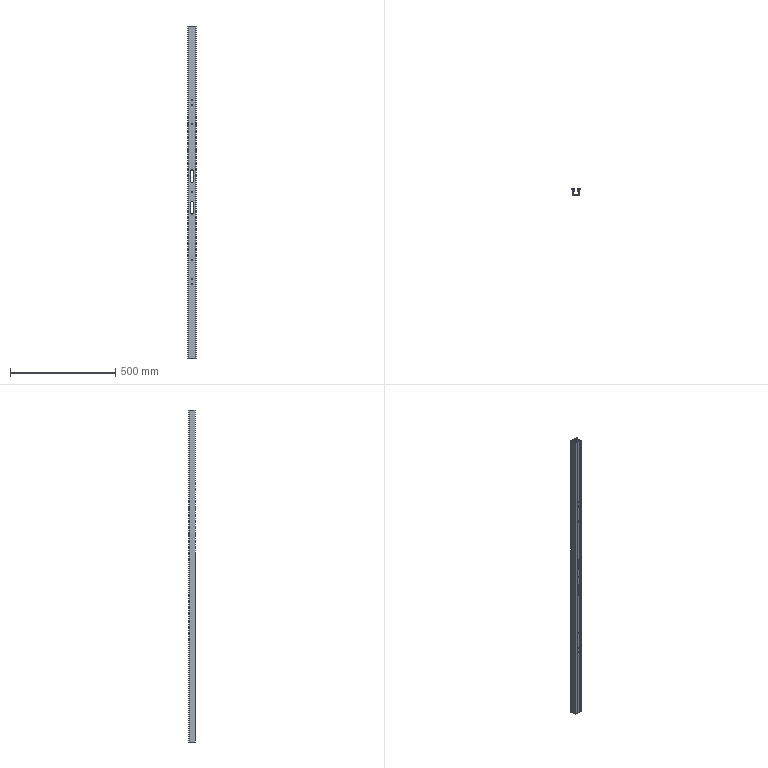Part | 2 solids | 118 faces | box 40 x 30 x 1580 mm | volume 535607 mm3 | plane 62 | cylinder 56 | commonest cylinder face diameters 6 x28 2 x14 11 x12 3 x2